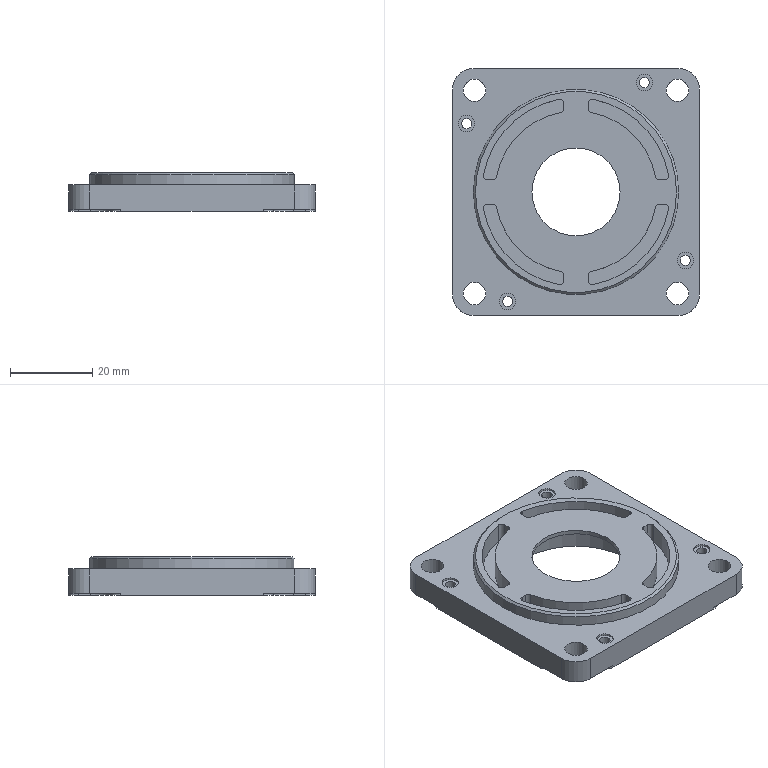Part | STEP file | 1 solid | 92 faces | box 60.2 x 60.2 x 9.5 mm | volume 18131 mm3 | cylinder 55 | plane 36 | cone 1 | commonest cylinder face diameters 2 x16 5 x8 10 x8 2.5 x4 4 x4 5.5 x4